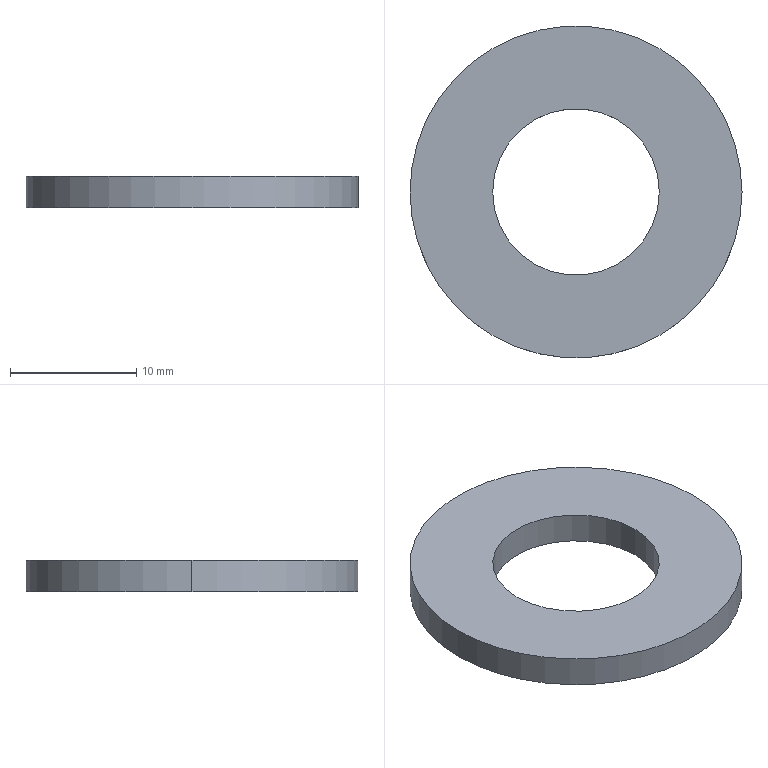Part | SolidWorks | features Extrusion 1 | 1 solid | 6 faces | box 26.3 x 26.3 x 2.5 mm | volume 1016 mm3 | cylinder 4 | plane 2 | commonest cylinder face diameters 13.2 x2 26.3 x2
STEP:
#1=CARTESIAN_POINT('',(-6.6,0.,1.25));
#2=VERTEX_POINT('',#1);
#3=CARTESIAN_POINT('',(6.6,0.,1.25));
#4=VERTEX_POINT('',#3);
#5=CARTESIAN_POINT('',(0.,0.,1.25));
#6=DIRECTION('',(0.,0.,1.));
#7=DIRECTION('',(1.,0.,0.));
#8=AXIS2_PLACEMENT_3D('',#5,#6,#7);
#9=CIRCLE('',#8,6.6);
#10=EDGE_CURVE('',#2,#4,#9,.T.);
#11=ORIENTED_EDGE('',*,*,#10,.T.);
#12=CARTESIAN_POINT('',(6.6,0.,-1.25));
#13=VERTEX_POINT('',#12);
#14=CARTESIAN_POINT('',(6.6,0.,1.25));
#15=DIRECTION('',(0.,0.,-1.));
#16=VECTOR('',#15,1000.);
#17=LINE('',#14,#16);
#18=EDGE_CURVE('',#4,#13,#17,.T.);
#19=ORIENTED_EDGE('',*,*,#18,.T.);
#20=CARTESIAN_POINT('',(-6.6,0.,-1.25));
#21=VERTEX_POINT('',#20);
#22=CARTESIAN_POINT('',(0.,0.,-1.25));
#23=DIRECTION('',(0.,0.,1.));
#24=DIRECTION('',(1.,0.,0.));
#25=AXIS2_PLACEMENT_3D('',#22,#23,#24);
#26=CIRCLE('',#25,6.6);
#27=EDGE_CURVE('',#21,#13,#26,.T.);
#28=ORIENTED_EDGE('',*,*,#27,.F.);
#29=CARTESIAN_POINT('',(-6.6,0.,1.25));
#30=DIRECTION('',(0.,0.,-1.));
#31=VECTOR('',#30,1000.);
#32=LINE('',#29,#31);
#33=EDGE_CURVE('',#2,#21,#32,.T.);
#34=ORIENTED_EDGE('',*,*,#33,.F.);
#35=EDGE_LOOP('',(#11,#19,#28,#34));
#36=FACE_OUTER_BOUND('',#35,.T.);
#37=CARTESIAN_POINT('',(0.,0.,1.25));
#38=DIRECTION('',(0.,0.,-1.));
#39=DIRECTION('',(-1.,0.,0.));
#40=AXIS2_PLACEMENT_3D('',#37,#38,#39);
#41=CYLINDRICAL_SURFACE('',#40,6.6);
#42=ADVANCED_FACE('',(#36),#41,.F.);
#43=CARTESIAN_POINT('',(13.15,0.,1.25));
#44=VERTEX_POINT('',#43);
#45=CARTESIAN_POINT('',(-13.15,0.,1.25));
#46=VERTEX_POINT('',#45);
#47=CARTESIAN_POINT('',(0.,0.,1.25));
#48=DIRECTION('',(0.,0.,1.));
#49=DIRECTION('',(1.,0.,0.));
#50=AXIS2_PLACEMENT_3D('',#47,#48,#49);
#51=CIRCLE('',#50,13.15);
#52=EDGE_CURVE('',#44,#46,#51,.T.);
#53=ORIENTED_EDGE('',*,*,#52,.F.);
#54=CARTESIAN_POINT('',(13.15,0.,-1.25));
#55=VERTEX_POINT('',#54);
#56=CARTESIAN_POINT('',(13.15,0.,1.25));
#57=DIRECTION('',(0.,0.,-1.));
#58=VECTOR('',#57,1000.);
#59=LINE('',#56,#58);
#60=EDGE_CURVE('',#44,#55,#59,.T.);
#61=ORIENTED_EDGE('',*,*,#60,.T.);
#62=CARTESIAN_POINT('',(-13.15,0.,-1.25));
#63=VERTEX_POINT('',#62);
#64=CARTESIAN_POINT('',(0.,0.,-1.25));
#65=DIRECTION('',(0.,0.,1.));
#66=DIRECTION('',(1.,0.,0.));
#67=AXIS2_PLACEMENT_3D('',#64,#65,#66);
#68=CIRCLE('',#67,13.15);
#69=EDGE_CURVE('',#55,#63,#68,.T.);
#70=ORIENTED_EDGE('',*,*,#69,.T.);
#71=CARTESIAN_POINT('',(-13.15,0.,1.25));
#72=DIRECTION('',(0.,0.,-1.));
#73=VECTOR('',#72,1000.);
#74=LINE('',#71,#73);
#75=EDGE_CURVE('',#46,#63,#74,.T.);
#76=ORIENTED_EDGE('',*,*,#75,.F.);
#77=EDGE_LOOP('',(#53,#61,#70,#76));
#78=FACE_OUTER_BOUND('',#77,.T.);
#79=CARTESIAN_POINT('',(0.,0.,1.25));
#80=DIRECTION('',(0.,0.,-1.));
#81=DIRECTION('',(-1.,0.,0.));
#82=AXIS2_PLACEMENT_3D('',#79,#80,#81);
#83=CYLINDRICAL_SURFACE('',#82,13.15);
#84=ADVANCED_FACE('',(#78),#83,.T.);
#85=CARTESIAN_POINT('',(0.,0.,1.25));
#86=DIRECTION('',(0.,0.,1.));
#87=DIRECTION('',(1.,0.,0.));
#88=AXIS2_PLACEMENT_3D('',#85,#86,#87);
#89=CIRCLE('',#88,13.15);
#90=EDGE_CURVE('',#46,#44,#89,.T.);
#91=ORIENTED_EDGE('',*,*,#90,.T.);
#92=ORIENTED_EDGE('',*,*,#52,.T.);
#93=EDGE_LOOP('',(#91,#92));
#94=FACE_OUTER_BOUND('',#93,.T.);
#95=ORIENTED_EDGE('',*,*,#10,.F.);
#96=CARTESIAN_POINT('',(0.,0.,1.25));
#97=DIRECTION('',(0.,0.,1.));
#98=DIRECTION('',(1.,0.,0.));
#99=AXIS2_PLACEMENT_3D('',#96,#97,#98);
#100=CIRCLE('',#99,6.6);
#101=EDGE_CURVE('',#4,#2,#100,.T.);
#102=ORIENTED_EDGE('',*,*,#101,.F.);
#103=EDGE_LOOP('',(#95,#102));
#104=FACE_BOUND('',#103,.T.);
#105=CARTESIAN_POINT('',(0.,0.,1.25));
#106=DIRECTION('',(0.,0.,1.));
#107=DIRECTION('',(1.,0.,0.));
#108=AXIS2_PLACEMENT_3D('',#105,#106,#107);
#109=PLANE('',#108);
#110=ADVANCED_FACE('',(#94,#104),#109,.T.);
#111=CARTESIAN_POINT('',(0.,0.,-1.25));
#112=DIRECTION('',(0.,0.,1.));
#113=DIRECTION('',(1.,0.,0.));
#114=AXIS2_PLACEMENT_3D('',#111,#112,#113);
#115=CIRCLE('',#114,13.15);
#116=EDGE_CURVE('',#63,#55,#115,.T.);
#117=ORIENTED_EDGE('',*,*,#116,.F.);
#118=ORIENTED_EDGE('',*,*,#69,.F.);
#119=EDGE_LOOP('',(#117,#118));
#120=FACE_OUTER_BOUND('',#119,.T.);
#121=ORIENTED_EDGE('',*,*,#27,.T.);
#122=CARTESIAN_POINT('',(0.,0.,-1.25));
#123=DIRECTION('',(0.,0.,1.));
#124=DIRECTION('',(1.,0.,0.));
#125=AXIS2_PLACEMENT_3D('',#122,#123,#124);
#126=CIRCLE('',#125,6.6);
#127=EDGE_CURVE('',#13,#21,#126,.T.);
#128=ORIENTED_EDGE('',*,*,#127,.T.);
#129=EDGE_LOOP('',(#121,#128));
#130=FACE_BOUND('',#129,.T.);
#131=CARTESIAN_POINT('',(0.,0.,-1.25));
#132=DIRECTION('',(0.,0.,1.));
#133=DIRECTION('',(1.,0.,0.));
#134=AXIS2_PLACEMENT_3D('',#131,#132,#133);
#135=PLANE('',#134);
#136=ADVANCED_FACE('',(#120,#130),#135,.F.);
#137=ORIENTED_EDGE('',*,*,#60,.F.);
#138=ORIENTED_EDGE('',*,*,#90,.F.);
#139=ORIENTED_EDGE('',*,*,#75,.T.);
#140=ORIENTED_EDGE('',*,*,#116,.T.);
#141=EDGE_LOOP('',(#137,#138,#139,#140));
#142=FACE_OUTER_BOUND('',#141,.T.);
#143=CARTESIAN_POINT('',(0.,0.,1.25));
#144=DIRECTION('',(0.,0.,-1.));
#145=DIRECTION('',(-1.,0.,0.));
#146=AXIS2_PLACEMENT_3D('',#143,#144,#145);
#147=CYLINDRICAL_SURFACE('',#146,13.15);
#148=ADVANCED_FACE('',(#142),#147,.T.);
#149=ORIENTED_EDGE('',*,*,#18,.F.);
#150=ORIENTED_EDGE('',*,*,#101,.T.);
#151=ORIENTED_EDGE('',*,*,#33,.T.);
#152=ORIENTED_EDGE('',*,*,#127,.F.);
#153=EDGE_LOOP('',(#149,#150,#151,#152));
#154=FACE_OUTER_BOUND('',#153,.T.);
#155=CARTESIAN_POINT('',(0.,0.,1.25));
#156=DIRECTION('',(0.,0.,-1.));
#157=DIRECTION('',(-1.,0.,0.));
#158=AXIS2_PLACEMENT_3D('',#155,#156,#157);
#159=CYLINDRICAL_SURFACE('',#158,6.6);
#160=ADVANCED_FACE('',(#154),#159,.F.);
#161=CLOSED_SHELL('',(#42,#84,#110,#136,#148,#160));
#162=MANIFOLD_SOLID_BREP('',#161);
#163=CARTESIAN_POINT('',(0.,0.,0.));
#164=DIRECTION('',(0.,0.,1.));
#165=DIRECTION('',(1.,0.,0.));
#166=AXIS2_PLACEMENT_3D('',#163,#164,#165);
#167=(LENGTH_UNIT()NAMED_UNIT(*)SI_UNIT(.MILLI.,.METRE.));
#168=UNCERTAINTY_MEASURE_WITH_UNIT(LENGTH_MEASURE(0.00001),#167,'','');
#169=(NAMED_UNIT(*)PLANE_ANGLE_UNIT()SI_UNIT($,.RADIAN.));
#170=(NAMED_UNIT(*)SI_UNIT($,.STERADIAN.)SOLID_ANGLE_UNIT());
#171=(GEOMETRIC_REPRESENTATION_CONTEXT(3)GLOBAL_UNCERTAINTY_ASSIGNED_CONTEXT((#168))GLOBAL_UNIT_ASSIGNED_CONTEXT((#167,#169,#170))REPRESENTATION_CONTEXT('',''));
#172=ADVANCED_BREP_SHAPE_REPRESENTATION('',(#162,#166),#171);